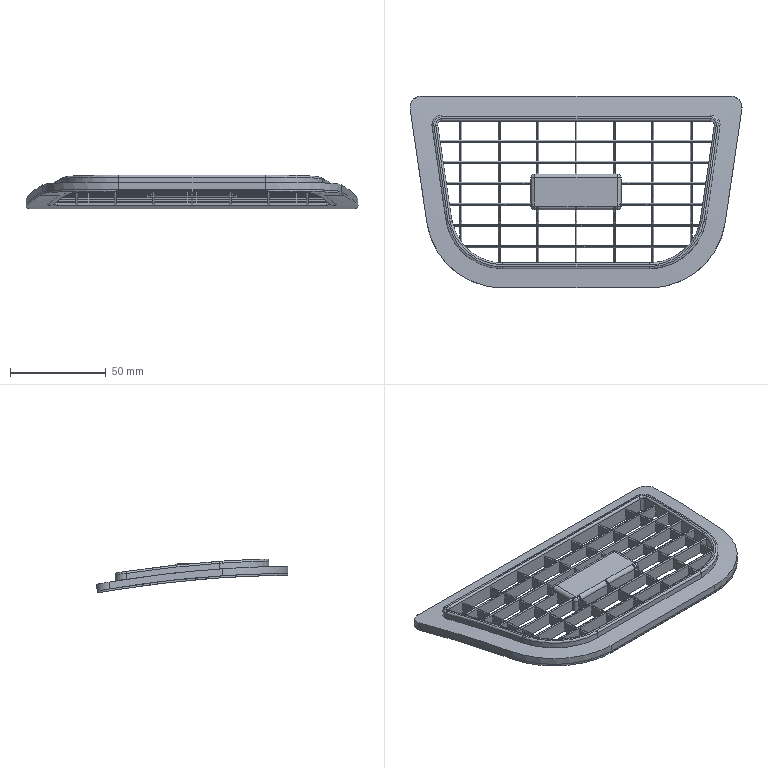Part | SolidWorks | features ICE 12, Fillet 3, Extrusion 1 | 3 solids | 377 faces | box 173.097 x 100 x 17.606 mm | volume 46536 mm3 | plane 158 | spline 144 | cylinder 71 | sphere 4 | commonest cylinder face diameters 1 x16 4 x14 54 x10 10 x9 12 x6 2 x4